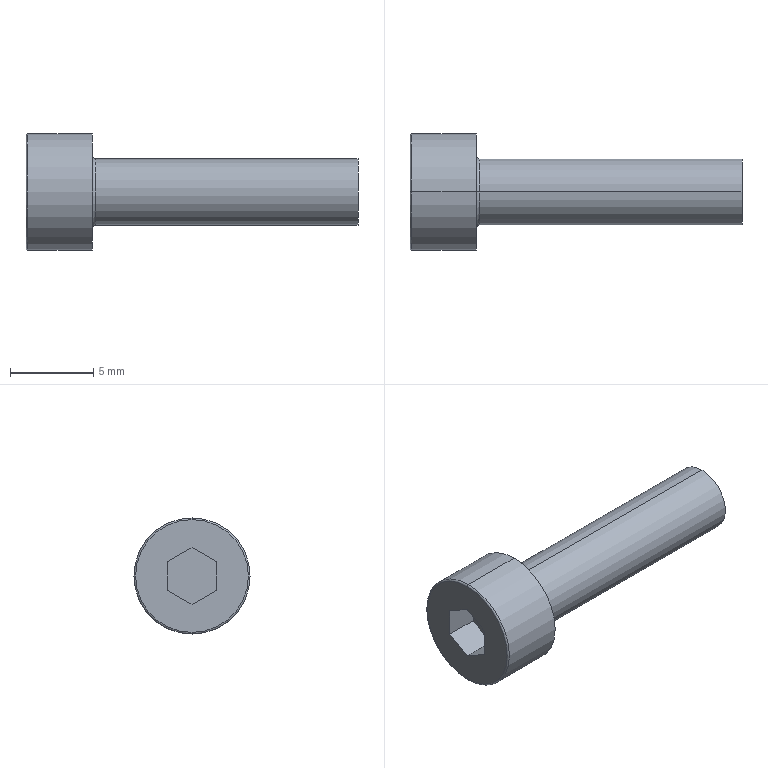Part | SolidWorks | features BlendCut 1, Cut 1, Fillet 1, LPattern 1, RevCut 1, Revolution 1 | 1 solid | 18 faces | box 20 x 7 x 7 mm | volume 339.691 mm3 | plane 10 | torus 4 | cylinder 4 | commonest cylinder face diameters 4 x2 7 x2
STEP:
#1=CARTESIAN_POINT('',(0.,0.,3.4));
#2=VERTEX_POINT('',#1);
#3=CARTESIAN_POINT('',(0.,0.,-3.4));
#4=VERTEX_POINT('',#3);
#5=CARTESIAN_POINT('',(0.,0.,0.));
#6=DIRECTION('',(-1.,0.,0.));
#7=DIRECTION('',(0.,0.,-1.));
#8=AXIS2_PLACEMENT_3D('',#5,#6,#7);
#9=CIRCLE('',#8,3.4);
#10=EDGE_CURVE('',#2,#4,#9,.T.);
#11=ORIENTED_EDGE('',*,*,#10,.F.);
#12=CARTESIAN_POINT('',(0.1,0.,3.5));
#13=VERTEX_POINT('',#12);
#14=CARTESIAN_POINT('',(0.1,0.,3.4));
#15=DIRECTION('',(0.,1.,0.));
#16=DIRECTION('',(0.,0.,1.));
#17=AXIS2_PLACEMENT_3D('',#14,#15,#16);
#18=CIRCLE('',#17,0.1);
#19=EDGE_CURVE('',#2,#13,#18,.T.);
#20=ORIENTED_EDGE('',*,*,#19,.T.);
#21=CARTESIAN_POINT('',(0.1,0.,-3.5));
#22=VERTEX_POINT('',#21);
#23=CARTESIAN_POINT('',(0.1,0.,0.));
#24=DIRECTION('',(1.,0.,0.));
#25=DIRECTION('',(0.,0.,-1.));
#26=AXIS2_PLACEMENT_3D('',#23,#24,#25);
#27=CIRCLE('',#26,3.5);
#28=EDGE_CURVE('',#22,#13,#27,.T.);
#29=ORIENTED_EDGE('',*,*,#28,.F.);
#30=CARTESIAN_POINT('',(0.1,0.,-3.4));
#31=DIRECTION('',(0.,-1.,0.));
#32=DIRECTION('',(0.,0.,-1.));
#33=AXIS2_PLACEMENT_3D('',#30,#31,#32);
#34=CIRCLE('',#33,0.1);
#35=EDGE_CURVE('',#4,#22,#34,.T.);
#36=ORIENTED_EDGE('',*,*,#35,.F.);
#37=EDGE_LOOP('',(#11,#20,#29,#36));
#38=FACE_OUTER_BOUND('',#37,.T.);
#39=CARTESIAN_POINT('',(0.1,0.,0.));
#40=DIRECTION('',(1.,0.,0.));
#41=DIRECTION('',(0.,0.,-1.));
#42=AXIS2_PLACEMENT_3D('',#39,#40,#41);
#43=TOROIDAL_SURFACE('',#42,3.4,0.1);
#44=ADVANCED_FACE('',(#38),#43,.T.);
#45=CARTESIAN_POINT('',(20.,0.,2.));
#46=VERTEX_POINT('',#45);
#47=CARTESIAN_POINT('',(20.,0.,-2.));
#48=VERTEX_POINT('',#47);
#49=CARTESIAN_POINT('',(20.,0.,0.));
#50=DIRECTION('',(-1.,0.,0.));
#51=DIRECTION('',(0.,0.,1.));
#52=AXIS2_PLACEMENT_3D('',#49,#50,#51);
#53=CIRCLE('',#52,2.);
#54=EDGE_CURVE('',#46,#48,#53,.T.);
#55=ORIENTED_EDGE('',*,*,#54,.T.);
#56=CARTESIAN_POINT('',(4.2,0.,-2.));
#57=VERTEX_POINT('',#56);
#58=CARTESIAN_POINT('',(0.,0.,-2.));
#59=DIRECTION('',(-1.,0.,0.));
#60=VECTOR('',#59,1000.);
#61=LINE('',#58,#60);
#62=EDGE_CURVE('',#48,#57,#61,.T.);
#63=ORIENTED_EDGE('',*,*,#62,.T.);
#64=CARTESIAN_POINT('',(4.2,0.,2.));
#65=VERTEX_POINT('',#64);
#66=CARTESIAN_POINT('',(4.2,0.,0.));
#67=DIRECTION('',(-1.,0.,0.));
#68=DIRECTION('',(0.,0.,1.));
#69=AXIS2_PLACEMENT_3D('',#66,#67,#68);
#70=CIRCLE('',#69,2.);
#71=EDGE_CURVE('',#65,#57,#70,.T.);
#72=ORIENTED_EDGE('',*,*,#71,.F.);
#73=CARTESIAN_POINT('',(0.,0.,2.));
#74=DIRECTION('',(-1.,0.,0.));
#75=VECTOR('',#74,1000.);
#76=LINE('',#73,#75);
#77=EDGE_CURVE('',#46,#65,#76,.T.);
#78=ORIENTED_EDGE('',*,*,#77,.F.);
#79=EDGE_LOOP('',(#55,#63,#72,#78));
#80=FACE_OUTER_BOUND('',#79,.T.);
#81=CARTESIAN_POINT('',(0.,0.,0.));
#82=DIRECTION('',(-1.,0.,0.));
#83=DIRECTION('',(0.,0.,1.));
#84=AXIS2_PLACEMENT_3D('',#81,#82,#83);
#85=CYLINDRICAL_SURFACE('',#84,2.);
#86=ADVANCED_FACE('',(#80),#85,.T.);
#87=CARTESIAN_POINT('',(4.,0.,-2.2));
#88=VERTEX_POINT('',#87);
#89=CARTESIAN_POINT('',(4.,0.,2.2));
#90=VERTEX_POINT('',#89);
#91=CARTESIAN_POINT('',(4.,0.,0.));
#92=DIRECTION('',(-1.,0.,0.));
#93=DIRECTION('',(0.,0.,1.));
#94=AXIS2_PLACEMENT_3D('',#91,#92,#93);
#95=CIRCLE('',#94,2.2);
#96=EDGE_CURVE('',#88,#90,#95,.T.);
#97=ORIENTED_EDGE('',*,*,#96,.F.);
#98=CARTESIAN_POINT('',(4.2,0.,-2.2));
#99=DIRECTION('',(0.,1.,0.));
#100=DIRECTION('',(0.,0.,1.));
#101=AXIS2_PLACEMENT_3D('',#98,#99,#100);
#102=CIRCLE('',#101,0.2);
#103=EDGE_CURVE('',#88,#57,#102,.T.);
#104=ORIENTED_EDGE('',*,*,#103,.T.);
#105=CARTESIAN_POINT('',(4.2,0.,0.));
#106=DIRECTION('',(-1.,0.,0.));
#107=DIRECTION('',(0.,0.,1.));
#108=AXIS2_PLACEMENT_3D('',#105,#106,#107);
#109=CIRCLE('',#108,2.);
#110=EDGE_CURVE('',#57,#65,#109,.T.);
#111=ORIENTED_EDGE('',*,*,#110,.T.);
#112=CARTESIAN_POINT('',(4.2,0.,2.2));
#113=DIRECTION('',(0.,-1.,0.));
#114=DIRECTION('',(0.,0.,-1.));
#115=AXIS2_PLACEMENT_3D('',#112,#113,#114);
#116=CIRCLE('',#115,0.2);
#117=EDGE_CURVE('',#90,#65,#116,.T.);
#118=ORIENTED_EDGE('',*,*,#117,.F.);
#119=EDGE_LOOP('',(#97,#104,#111,#118));
#120=FACE_OUTER_BOUND('',#119,.T.);
#121=CARTESIAN_POINT('',(4.2,0.,0.));
#122=DIRECTION('',(-1.,0.,0.));
#123=DIRECTION('',(0.,0.,1.));
#124=AXIS2_PLACEMENT_3D('',#121,#122,#123);
#125=TOROIDAL_SURFACE('',#124,2.2,0.2);
#126=ADVANCED_FACE('',(#120),#125,.F.);
#127=CARTESIAN_POINT('',(4.,0.,3.5));
#128=VERTEX_POINT('',#127);
#129=CARTESIAN_POINT('',(4.,0.,-3.5));
#130=VERTEX_POINT('',#129);
#131=CARTESIAN_POINT('',(4.,0.,0.));
#132=DIRECTION('',(-1.,0.,0.));
#133=DIRECTION('',(0.,0.,1.));
#134=AXIS2_PLACEMENT_3D('',#131,#132,#133);
#135=CIRCLE('',#134,3.5);
#136=EDGE_CURVE('',#128,#130,#135,.T.);
#137=ORIENTED_EDGE('',*,*,#136,.T.);
#138=CARTESIAN_POINT('',(0.,0.,-3.5));
#139=DIRECTION('',(-1.,0.,0.));
#140=VECTOR('',#139,1000.);
#141=LINE('',#138,#140);
#142=EDGE_CURVE('',#130,#22,#141,.T.);
#143=ORIENTED_EDGE('',*,*,#142,.T.);
#144=ORIENTED_EDGE('',*,*,#28,.T.);
#145=CARTESIAN_POINT('',(0.,0.,3.5));
#146=DIRECTION('',(-1.,0.,0.));
#147=VECTOR('',#146,1000.);
#148=LINE('',#145,#147);
#149=EDGE_CURVE('',#128,#13,#148,.T.);
#150=ORIENTED_EDGE('',*,*,#149,.F.);
#151=EDGE_LOOP('',(#137,#143,#144,#150));
#152=FACE_OUTER_BOUND('',#151,.T.);
#153=CARTESIAN_POINT('',(0.,0.,0.));
#154=DIRECTION('',(-1.,0.,0.));
#155=DIRECTION('',(0.,0.,1.));
#156=AXIS2_PLACEMENT_3D('',#153,#154,#155);
#157=CYLINDRICAL_SURFACE('',#156,3.5);
#158=ADVANCED_FACE('',(#152),#157,.T.);
#159=CARTESIAN_POINT('',(0.,0.,0.));
#160=DIRECTION('',(-1.,0.,0.));
#161=DIRECTION('',(0.,0.,-1.));
#162=AXIS2_PLACEMENT_3D('',#159,#160,#161);
#163=CIRCLE('',#162,3.4);
#164=EDGE_CURVE('',#4,#2,#163,.T.);
#165=ORIENTED_EDGE('',*,*,#164,.T.);
#166=ORIENTED_EDGE('',*,*,#10,.T.);
#167=EDGE_LOOP('',(#165,#166));
#168=FACE_OUTER_BOUND('',#167,.T.);
#169=CARTESIAN_POINT('',(0.,0.,1.72));
#170=VERTEX_POINT('',#169);
#171=CARTESIAN_POINT('',(0.,1.49,0.86));
#172=VERTEX_POINT('',#171);
#173=CARTESIAN_POINT('',(0.,0.,1.72));
#174=DIRECTION('',(0.,0.866,-0.5));
#175=VECTOR('',#174,1000.);
#176=LINE('',#173,#175);
#177=EDGE_CURVE('',#170,#172,#176,.T.);
#178=ORIENTED_EDGE('',*,*,#177,.F.);
#179=CARTESIAN_POINT('',(0.,-1.49,0.86));
#180=VERTEX_POINT('',#179);
#181=CARTESIAN_POINT('',(0.,-1.49,0.86));
#182=DIRECTION('',(0.,0.866,0.5));
#183=VECTOR('',#182,1000.);
#184=LINE('',#181,#183);
#185=EDGE_CURVE('',#180,#170,#184,.T.);
#186=ORIENTED_EDGE('',*,*,#185,.F.);
#187=CARTESIAN_POINT('',(0.,-1.49,-0.86));
#188=VERTEX_POINT('',#187);
#189=CARTESIAN_POINT('',(0.,-1.49,-0.86));
#190=DIRECTION('',(0.,0.,1.));
#191=VECTOR('',#190,1000.);
#192=LINE('',#189,#191);
#193=EDGE_CURVE('',#188,#180,#192,.T.);
#194=ORIENTED_EDGE('',*,*,#193,.F.);
#195=CARTESIAN_POINT('',(0.,0.,-1.72));
#196=VERTEX_POINT('',#195);
#197=CARTESIAN_POINT('',(0.,0.,-1.72));
#198=DIRECTION('',(0.,-0.866,0.5));
#199=VECTOR('',#198,1000.);
#200=LINE('',#197,#199);
#201=EDGE_CURVE('',#196,#188,#200,.T.);
#202=ORIENTED_EDGE('',*,*,#201,.F.);
#203=CARTESIAN_POINT('',(0.,1.49,-0.86));
#204=VERTEX_POINT('',#203);
#205=CARTESIAN_POINT('',(0.,1.49,-0.86));
#206=DIRECTION('',(0.,-0.866,-0.5));
#207=VECTOR('',#206,1000.);
#208=LINE('',#205,#207);
#209=EDGE_CURVE('',#204,#196,#208,.T.);
#210=ORIENTED_EDGE('',*,*,#209,.F.);
#211=CARTESIAN_POINT('',(0.,1.49,0.86));
#212=DIRECTION('',(0.,0.,-1.));
#213=VECTOR('',#212,1000.);
#214=LINE('',#211,#213);
#215=EDGE_CURVE('',#172,#204,#214,.T.);
#216=ORIENTED_EDGE('',*,*,#215,.F.);
#217=EDGE_LOOP('',(#178,#186,#194,#202,#210,#216));
#218=FACE_BOUND('',#217,.T.);
#219=CARTESIAN_POINT('',(0.,0.,0.));
#220=DIRECTION('',(1.,0.,0.));
#221=DIRECTION('',(0.,0.,-1.));
#222=AXIS2_PLACEMENT_3D('',#219,#220,#221);
#223=PLANE('',#222);
#224=ADVANCED_FACE('',(#168,#218),#223,.F.);
#225=ORIENTED_EDGE('',*,*,#142,.F.);
#226=CARTESIAN_POINT('',(4.,0.,0.));
#227=DIRECTION('',(-1.,0.,0.));
#228=DIRECTION('',(0.,0.,1.));
#229=AXIS2_PLACEMENT_3D('',#226,#227,#228);
#230=CIRCLE('',#229,3.5);
#231=EDGE_CURVE('',#130,#128,#230,.T.);
#232=ORIENTED_EDGE('',*,*,#231,.T.);
#233=ORIENTED_EDGE('',*,*,#149,.T.);
#234=CARTESIAN_POINT('',(0.1,0.,0.));
#235=DIRECTION('',(1.,0.,0.));
#236=DIRECTION('',(0.,0.,-1.));
#237=AXIS2_PLACEMENT_3D('',#234,#235,#236);
#238=CIRCLE('',#237,3.5);
#239=EDGE_CURVE('',#13,#22,#238,.T.);
#240=ORIENTED_EDGE('',*,*,#239,.T.);
#241=EDGE_LOOP('',(#225,#232,#233,#240));
#242=FACE_OUTER_BOUND('',#241,.T.);
#243=CARTESIAN_POINT('',(0.,0.,0.));
#244=DIRECTION('',(-1.,0.,0.));
#245=DIRECTION('',(0.,0.,1.));
#246=AXIS2_PLACEMENT_3D('',#243,#244,#245);
#247=CYLINDRICAL_SURFACE('',#246,3.5);
#248=ADVANCED_FACE('',(#242),#247,.T.);
#249=ORIENTED_EDGE('',*,*,#136,.F.);
#250=ORIENTED_EDGE('',*,*,#231,.F.);
#251=EDGE_LOOP('',(#249,#250));
#252=FACE_OUTER_BOUND('',#251,.T.);
#253=CARTESIAN_POINT('',(4.,0.,0.));
#254=DIRECTION('',(-1.,0.,0.));
#255=DIRECTION('',(0.,0.,1.));
#256=AXIS2_PLACEMENT_3D('',#253,#254,#255);
#257=CIRCLE('',#256,2.2);
#258=EDGE_CURVE('',#90,#88,#257,.T.);
#259=ORIENTED_EDGE('',*,*,#258,.T.);
#260=ORIENTED_EDGE('',*,*,#96,.T.);
#261=EDGE_LOOP('',(#259,#260));
#262=FACE_BOUND('',#261,.T.);
#263=CARTESIAN_POINT('',(4.,3.5,0.));
#264=DIRECTION('',(-1.,0.,0.));
#265=DIRECTION('',(0.,0.,1.));
#266=AXIS2_PLACEMENT_3D('',#263,#264,#265);
#267=PLANE('',#266);
#268=ADVANCED_FACE('',(#252,#262),#267,.F.);
#269=ORIENTED_EDGE('',*,*,#103,.F.);
#270=ORIENTED_EDGE('',*,*,#258,.F.);
#271=ORIENTED_EDGE('',*,*,#117,.T.);
#272=ORIENTED_EDGE('',*,*,#71,.T.);
#273=EDGE_LOOP('',(#269,#270,#271,#272));
#274=FACE_OUTER_BOUND('',#273,.T.);
#275=CARTESIAN_POINT('',(4.2,0.,0.));
#276=DIRECTION('',(-1.,0.,0.));
#277=DIRECTION('',(0.,0.,1.));
#278=AXIS2_PLACEMENT_3D('',#275,#276,#277);
#279=TOROIDAL_SURFACE('',#278,2.2,0.2);
#280=ADVANCED_FACE('',(#274),#279,.F.);
#281=ORIENTED_EDGE('',*,*,#62,.F.);
#282=CARTESIAN_POINT('',(20.,0.,0.));
#283=DIRECTION('',(-1.,0.,0.));
#284=DIRECTION('',(0.,0.,1.));
#285=AXIS2_PLACEMENT_3D('',#282,#283,#284);
#286=CIRCLE('',#285,2.);
#287=EDGE_CURVE('',#48,#46,#286,.T.);
#288=ORIENTED_EDGE('',*,*,#287,.T.);
#289=ORIENTED_EDGE('',*,*,#77,.T.);
#290=ORIENTED_EDGE('',*,*,#110,.F.);
#291=EDGE_LOOP('',(#281,#288,#289,#290));
#292=FACE_OUTER_BOUND('',#291,.T.);
#293=CARTESIAN_POINT('',(0.,0.,0.));
#294=DIRECTION('',(-1.,0.,0.));
#295=DIRECTION('',(0.,0.,1.));
#296=AXIS2_PLACEMENT_3D('',#293,#294,#295);
#297=CYLINDRICAL_SURFACE('',#296,2.);
#298=ADVANCED_FACE('',(#292),#297,.T.);
#299=ORIENTED_EDGE('',*,*,#54,.F.);
#300=ORIENTED_EDGE('',*,*,#287,.F.);
#301=EDGE_LOOP('',(#299,#300));
#302=FACE_OUTER_BOUND('',#301,.T.);
#303=CARTESIAN_POINT('',(20.,2.,0.));
#304=DIRECTION('',(-1.,0.,0.));
#305=DIRECTION('',(0.,0.,1.));
#306=AXIS2_PLACEMENT_3D('',#303,#304,#305);
#307=PLANE('',#306);
#308=ADVANCED_FACE('',(#302),#307,.F.);
#309=ORIENTED_EDGE('',*,*,#185,.T.);
#310=CARTESIAN_POINT('',(2.,0.,1.72));
#311=VERTEX_POINT('',#310);
#312=CARTESIAN_POINT('',(2.,0.,1.72));
#313=DIRECTION('',(-1.,0.,0.));
#314=VECTOR('',#313,1000.);
#315=LINE('',#312,#314);
#316=EDGE_CURVE('',#311,#170,#315,.T.);
#317=ORIENTED_EDGE('',*,*,#316,.F.);
#318=CARTESIAN_POINT('',(2.,-1.49,0.86));
#319=VERTEX_POINT('',#318);
#320=CARTESIAN_POINT('',(2.,-1.49,0.86));
#321=DIRECTION('',(0.,0.866,0.5));
#322=VECTOR('',#321,1000.);
#323=LINE('',#320,#322);
#324=EDGE_CURVE('',#319,#311,#323,.T.);
#325=ORIENTED_EDGE('',*,*,#324,.F.);
#326=CARTESIAN_POINT('',(2.,-1.49,0.86));
#327=DIRECTION('',(-1.,0.,0.));
#328=VECTOR('',#327,1000.);
#329=LINE('',#326,#328);
#330=EDGE_CURVE('',#319,#180,#329,.T.);
#331=ORIENTED_EDGE('',*,*,#330,.T.);
#332=EDGE_LOOP('',(#309,#317,#325,#331));
#333=FACE_OUTER_BOUND('',#332,.T.);
#334=CARTESIAN_POINT('',(2.,-1.49,0.86));
#335=DIRECTION('',(0.,-0.5,0.866));
#336=DIRECTION('',(0.,-0.866,-0.5));
#337=AXIS2_PLACEMENT_3D('',#334,#335,#336);
#338=PLANE('',#337);
#339=ADVANCED_FACE('',(#333),#338,.F.);
#340=ORIENTED_EDGE('',*,*,#193,.T.);
#341=ORIENTED_EDGE('',*,*,#330,.F.);
#342=CARTESIAN_POINT('',(2.,-1.49,-0.86));
#343=VERTEX_POINT('',#342);
#344=CARTESIAN_POINT('',(2.,-1.49,-0.86));
#345=DIRECTION('',(0.,0.,1.));
#346=VECTOR('',#345,1000.);
#347=LINE('',#344,#346);
#348=EDGE_CURVE('',#343,#319,#347,.T.);
#349=ORIENTED_EDGE('',*,*,#348,.F.);
#350=CARTESIAN_POINT('',(2.,-1.49,-0.86));
#351=DIRECTION('',(-1.,0.,0.));
#352=VECTOR('',#351,1000.);
#353=LINE('',#350,#352);
#354=EDGE_CURVE('',#343,#188,#353,.T.);
#355=ORIENTED_EDGE('',*,*,#354,.T.);
#356=EDGE_LOOP('',(#340,#341,#349,#355));
#357=FACE_OUTER_BOUND('',#356,.T.);
#358=CARTESIAN_POINT('',(2.,-1.49,-0.86));
#359=DIRECTION('',(0.,-1.,0.));
#360=DIRECTION('',(0.,0.,-1.));
#361=AXIS2_PLACEMENT_3D('',#358,#359,#360);
#362=PLANE('',#361);
#363=ADVANCED_FACE('',(#357),#362,.F.);
#364=ORIENTED_EDGE('',*,*,#201,.T.);
#365=ORIENTED_EDGE('',*,*,#354,.F.);
#366=CARTESIAN_POINT('',(2.,0.,-1.72));
#367=VERTEX_POINT('',#366);
#368=CARTESIAN_POINT('',(2.,0.,-1.72));
#369=DIRECTION('',(0.,-0.866,0.5));
#370=VECTOR('',#369,1000.);
#371=LINE('',#368,#370);
#372=EDGE_CURVE('',#367,#343,#371,.T.);
#373=ORIENTED_EDGE('',*,*,#372,.F.);
#374=CARTESIAN_POINT('',(2.,0.,-1.72));
#375=DIRECTION('',(-1.,0.,0.));
#376=VECTOR('',#375,1000.);
#377=LINE('',#374,#376);
#378=EDGE_CURVE('',#367,#196,#377,.T.);
#379=ORIENTED_EDGE('',*,*,#378,.T.);
#380=EDGE_LOOP('',(#364,#365,#373,#379));
#381=FACE_OUTER_BOUND('',#380,.T.);
#382=CARTESIAN_POINT('',(2.,0.,-1.72));
#383=DIRECTION('',(0.,-0.5,-0.866));
#384=DIRECTION('',(0.,0.866,-0.5));
#385=AXIS2_PLACEMENT_3D('',#382,#383,#384);
#386=PLANE('',#385);
#387=ADVANCED_FACE('',(#381),#386,.F.);
#388=ORIENTED_EDGE('',*,*,#209,.T.);
#389=ORIENTED_EDGE('',*,*,#378,.F.);
#390=CARTESIAN_POINT('',(2.,1.49,-0.86));
#391=VERTEX_POINT('',#390);
#392=CARTESIAN_POINT('',(2.,1.49,-0.86));
#393=DIRECTION('',(0.,-0.866,-0.5));
#394=VECTOR('',#393,1000.);
#395=LINE('',#392,#394);
#396=EDGE_CURVE('',#391,#367,#395,.T.);
#397=ORIENTED_EDGE('',*,*,#396,.F.);
#398=CARTESIAN_POINT('',(2.,1.49,-0.86));
#399=DIRECTION('',(-1.,0.,0.));
#400=VECTOR('',#399,1000.);
#401=LINE('',#398,#400);
#402=EDGE_CURVE('',#391,#204,#401,.T.);
#403=ORIENTED_EDGE('',*,*,#402,.T.);
#404=EDGE_LOOP('',(#388,#389,#397,#403));
#405=FACE_OUTER_BOUND('',#404,.T.);
#406=CARTESIAN_POINT('',(2.,1.49,-0.86));
#407=DIRECTION('',(0.,0.5,-0.866));
#408=DIRECTION('',(0.,0.866,0.5));
#409=AXIS2_PLACEMENT_3D('',#406,#407,#408);
#410=PLANE('',#409);
#411=ADVANCED_FACE('',(#405),#410,.F.);
#412=ORIENTED_EDGE('',*,*,#215,.T.);
#413=ORIENTED_EDGE('',*,*,#402,.F.);
#414=CARTESIAN_POINT('',(2.,1.49,0.86));
#415=VERTEX_POINT('',#414);
#416=CARTESIAN_POINT('',(2.,1.49,0.86));
#417=DIRECTION('',(0.,0.,-1.));
#418=VECTOR('',#417,1000.);
#419=LINE('',#416,#418);
#420=EDGE_CURVE('',#415,#391,#419,.T.);
#421=ORIENTED_EDGE('',*,*,#420,.F.);
#422=CARTESIAN_POINT('',(2.,1.49,0.86));
#423=DIRECTION('',(-1.,0.,0.));
#424=VECTOR('',#423,1000.);
#425=LINE('',#422,#424);
#426=EDGE_CURVE('',#415,#172,#425,.T.);
#427=ORIENTED_EDGE('',*,*,#426,.T.);
#428=EDGE_LOOP('',(#412,#413,#421,#427));
#429=FACE_OUTER_BOUND('',#428,.T.);
#430=CARTESIAN_POINT('',(2.,1.49,0.86));
#431=DIRECTION('',(0.,1.,0.));
#432=DIRECTION('',(0.,0.,1.));
#433=AXIS2_PLACEMENT_3D('',#430,#431,#432);
#434=PLANE('',#433);
#435=ADVANCED_FACE('',(#429),#434,.F.);
#436=ORIENTED_EDGE('',*,*,#177,.T.);
#437=ORIENTED_EDGE('',*,*,#426,.F.);
#438=CARTESIAN_POINT('',(2.,0.,1.72));
#439=DIRECTION('',(0.,0.866,-0.5));
#440=VECTOR('',#439,1000.);
#441=LINE('',#438,#440);
#442=EDGE_CURVE('',#311,#415,#441,.T.);
#443=ORIENTED_EDGE('',*,*,#442,.F.);
#444=ORIENTED_EDGE('',*,*,#316,.T.);
#445=EDGE_LOOP('',(#436,#437,#443,#444));
#446=FACE_OUTER_BOUND('',#445,.T.);
#447=CARTESIAN_POINT('',(2.,0.,1.72));
#448=DIRECTION('',(0.,0.5,0.866));
#449=DIRECTION('',(0.,-0.866,0.5));
#450=AXIS2_PLACEMENT_3D('',#447,#448,#449);
#451=PLANE('',#450);
#452=ADVANCED_FACE('',(#446),#451,.F.);
#453=ORIENTED_EDGE('',*,*,#324,.T.);
#454=ORIENTED_EDGE('',*,*,#442,.T.);
#455=ORIENTED_EDGE('',*,*,#420,.T.);
#456=ORIENTED_EDGE('',*,*,#396,.T.);
#457=ORIENTED_EDGE('',*,*,#372,.T.);
#458=ORIENTED_EDGE('',*,*,#348,.T.);
#459=EDGE_LOOP('',(#453,#454,#455,#456,#457,#458));
#460=FACE_OUTER_BOUND('',#459,.T.);
#461=CARTESIAN_POINT('',(2.,1.49,2.58));
#462=DIRECTION('',(-1.,0.,0.));
#463=DIRECTION('',(0.,0.,1.));
#464=AXIS2_PLACEMENT_3D('',#461,#462,#463);
#465=PLANE('',#464);
#466=ADVANCED_FACE('',(#460),#465,.T.);
#467=ORIENTED_EDGE('',*,*,#19,.F.);
#468=ORIENTED_EDGE('',*,*,#164,.F.);
#469=ORIENTED_EDGE('',*,*,#35,.T.);
#470=ORIENTED_EDGE('',*,*,#239,.F.);
#471=EDGE_LOOP('',(#467,#468,#469,#470));
#472=FACE_OUTER_BOUND('',#471,.T.);
#473=CARTESIAN_POINT('',(0.1,0.,0.));
#474=DIRECTION('',(1.,0.,0.));
#475=DIRECTION('',(0.,0.,-1.));
#476=AXIS2_PLACEMENT_3D('',#473,#474,#475);
#477=TOROIDAL_SURFACE('',#476,3.4,0.1);
#478=ADVANCED_FACE('',(#472),#477,.T.);
#479=CLOSED_SHELL('',(#44,#86,#126,#158,#224,#248,#268,#280,#298,#308,#339,#363,#387,#411,#435,#452,#466,#478));
#480=MANIFOLD_SOLID_BREP('',#479);
#481=CARTESIAN_POINT('',(0.,0.,0.));
#482=DIRECTION('',(0.,0.,1.));
#483=DIRECTION('',(1.,0.,0.));
#484=AXIS2_PLACEMENT_3D('',#481,#482,#483);
#485=(LENGTH_UNIT()NAMED_UNIT(*)SI_UNIT(.MILLI.,.METRE.));
#486=UNCERTAINTY_MEASURE_WITH_UNIT(LENGTH_MEASURE(0.00001),#485,'','');
#487=(NAMED_UNIT(*)PLANE_ANGLE_UNIT()SI_UNIT($,.RADIAN.));
#488=(NAMED_UNIT(*)SI_UNIT($,.STERADIAN.)SOLID_ANGLE_UNIT());
#489=(GEOMETRIC_REPRESENTATION_CONTEXT(3)GLOBAL_UNCERTAINTY_ASSIGNED_CONTEXT((#486))GLOBAL_UNIT_ASSIGNED_CONTEXT((#485,#487,#488))REPRESENTATION_CONTEXT('',''));
#490=ADVANCED_BREP_SHAPE_REPRESENTATION('',(#480,#484),#489);